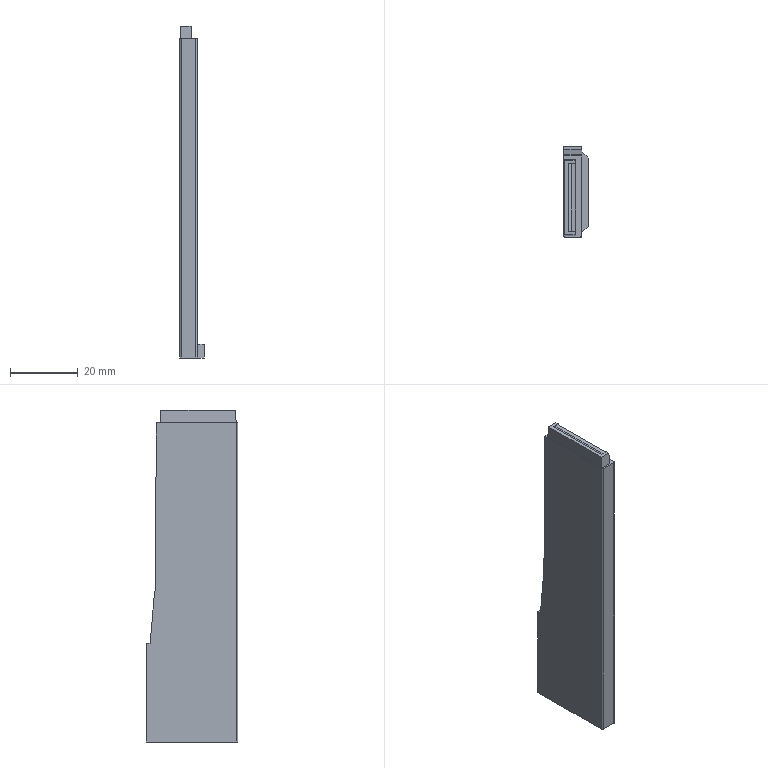Part | Creo | 1 solid | 28 faces | box 7.264 x 27.054 x 97.99 mm | volume 12954 mm3 | plane 25 | cylinder 3 | commonest cylinder face diameters 1 x3
STEP:
#1=CARTESIAN_POINT('',(0.,0.,0.));
#2=DIRECTION('',(0.,0.,1.));
#3=DIRECTION('',(1.,0.,0.));
#4=AXIS2_PLACEMENT_3D('',#1,#2,#3);
#5=CARTESIAN_POINT('',(19.635,62.146,-54.09));
#6=VERTEX_POINT('',#5);
#7=CARTESIAN_POINT('',(19.635,61.146,-54.09));
#8=VERTEX_POINT('',#7);
#9=CARTESIAN_POINT('',(19.635,62.146,-54.09));
#10=DIRECTION('',(0.,-1.,0.));
#11=VECTOR('',#10,1.);
#12=LINE('',#9,#11);
#13=EDGE_CURVE('',#6,#8,#12,.T.);
#14=ORIENTED_EDGE('',*,*,#13,.T.);
#15=CARTESIAN_POINT('',(19.635,61.146,40.081));
#16=VERTEX_POINT('',#15);
#17=CARTESIAN_POINT('',(19.635,61.146,-54.09));
#18=DIRECTION('',(0.,0.,1.));
#19=VECTOR('',#18,94.171);
#20=LINE('',#17,#19);
#21=EDGE_CURVE('',#8,#16,#20,.T.);
#22=ORIENTED_EDGE('',*,*,#21,.T.);
#23=CARTESIAN_POINT('',(19.635,84.661,40.081));
#24=VERTEX_POINT('',#23);
#25=CARTESIAN_POINT('',(19.635,61.146,40.081));
#26=DIRECTION('',(0.,1.,0.));
#27=VECTOR('',#26,23.515);
#28=LINE('',#25,#27);
#29=EDGE_CURVE('',#16,#24,#28,.T.);
#30=ORIENTED_EDGE('',*,*,#29,.T.);
#31=CARTESIAN_POINT('',(19.635,85.096,-9.767));
#32=VERTEX_POINT('',#31);
#33=CARTESIAN_POINT('',(19.635,85.096,-9.767));
#34=DIRECTION('',(0.,-0.008727,1.));
#35=VECTOR('',#34,49.85);
#36=LINE('',#33,#35);
#37=EDGE_CURVE('',#32,#24,#36,.T.);
#38=ORIENTED_EDGE('',*,*,#37,.F.);
#39=CARTESIAN_POINT('',(19.635,85.218,-9.767));
#40=VERTEX_POINT('',#39);
#41=CARTESIAN_POINT('',(19.635,85.218,-9.767));
#42=DIRECTION('',(0.,-1.,0.));
#43=VECTOR('',#42,0.1217);
#44=LINE('',#41,#43);
#45=EDGE_CURVE('',#40,#32,#44,.T.);
#46=ORIENTED_EDGE('',*,*,#45,.F.);
#47=CARTESIAN_POINT('',(19.635,86.547,-24.967));
#48=VERTEX_POINT('',#47);
#49=CARTESIAN_POINT('',(19.635,86.547,-24.967));
#50=DIRECTION('',(0.,-0.08716,0.9962));
#51=VECTOR('',#50,15.258);
#52=LINE('',#49,#51);
#53=EDGE_CURVE('',#48,#40,#52,.T.);
#54=ORIENTED_EDGE('',*,*,#53,.F.);
#55=CARTESIAN_POINT('',(19.635,87.2,-24.967));
#56=VERTEX_POINT('',#55);
#57=CARTESIAN_POINT('',(19.635,87.2,-24.967));
#58=DIRECTION('',(0.,-1.,0.));
#59=VECTOR('',#58,0.6527);
#60=LINE('',#57,#59);
#61=EDGE_CURVE('',#56,#48,#60,.T.);
#62=ORIENTED_EDGE('',*,*,#61,.F.);
#63=CARTESIAN_POINT('',(19.635,87.2,-54.09));
#64=VERTEX_POINT('',#63);
#65=CARTESIAN_POINT('',(19.635,87.2,-24.967));
#66=DIRECTION('',(0.,0.,-1.));
#67=VECTOR('',#66,29.123);
#68=LINE('',#65,#67);
#69=EDGE_CURVE('',#56,#64,#68,.T.);
#70=ORIENTED_EDGE('',*,*,#69,.T.);
#71=CARTESIAN_POINT('',(19.635,86.2,-54.09));
#72=VERTEX_POINT('',#71);
#73=CARTESIAN_POINT('',(19.635,87.2,-54.09));
#74=DIRECTION('',(0.,-1.,0.));
#75=VECTOR('',#74,1.);
#76=LINE('',#73,#75);
#77=EDGE_CURVE('',#64,#72,#76,.T.);
#78=ORIENTED_EDGE('',*,*,#77,.T.);
#79=CARTESIAN_POINT('',(19.635,86.2,-50.09));
#80=VERTEX_POINT('',#79);
#81=CARTESIAN_POINT('',(19.635,86.2,-54.09));
#82=DIRECTION('',(0.,0.,1.));
#83=VECTOR('',#82,4.);
#84=LINE('',#81,#83);
#85=EDGE_CURVE('',#72,#80,#84,.T.);
#86=ORIENTED_EDGE('',*,*,#85,.T.);
#87=CARTESIAN_POINT('',(19.635,62.146,-50.09));
#88=VERTEX_POINT('',#87);
#89=CARTESIAN_POINT('',(19.635,86.2,-50.09));
#90=DIRECTION('',(0.,-1.,0.));
#91=VECTOR('',#90,24.054);
#92=LINE('',#89,#91);
#93=EDGE_CURVE('',#80,#88,#92,.T.);
#94=ORIENTED_EDGE('',*,*,#93,.T.);
#95=CARTESIAN_POINT('',(19.635,62.146,-50.09));
#96=DIRECTION('',(0.,0.,-1.));
#97=VECTOR('',#96,4.);
#98=LINE('',#95,#97);
#99=EDGE_CURVE('',#88,#6,#98,.T.);
#100=ORIENTED_EDGE('',*,*,#99,.T.);
#101=EDGE_LOOP('',(#14,#22,#30,#38,#46,#54,#62,#70,#78,#86,#94,#100));
#102=FACE_OUTER_BOUND('',#101,.F.);
#103=CARTESIAN_POINT('',(19.635,60.646,75.91));
#104=DIRECTION('',(-1.,0.,0.));
#105=DIRECTION('',(0.,-1.,0.));
#106=AXIS2_PLACEMENT_3D('',#103,#104,#105);
#107=PLANE('',#106);
#108=ADVANCED_FACE('',(#102),#107,.F.);
#109=ORIENTED_EDGE('',*,*,#77,.F.);
#110=CARTESIAN_POINT('',(19.135,87.7,-54.09));
#111=VERTEX_POINT('',#110);
#112=CARTESIAN_POINT('',(19.135,87.2,-54.09));
#113=DIRECTION('',(0.,0.,-1.));
#114=DIRECTION('',(0.,1.,0.));
#115=AXIS2_PLACEMENT_3D('',#112,#113,#114);
#116=CIRCLE('',#115,0.5);
#117=EDGE_CURVE('',#111,#64,#116,.T.);
#118=ORIENTED_EDGE('',*,*,#117,.F.);
#119=CARTESIAN_POINT('',(14.371,87.7,-54.09));
#120=VERTEX_POINT('',#119);
#121=CARTESIAN_POINT('',(14.371,87.7,-54.09));
#122=DIRECTION('',(1.,0.,0.));
#123=VECTOR('',#122,4.764);
#124=LINE('',#121,#123);
#125=EDGE_CURVE('',#120,#111,#124,.T.);
#126=ORIENTED_EDGE('',*,*,#125,.F.);
#127=CARTESIAN_POINT('',(14.371,61.146,-54.09));
#128=VERTEX_POINT('',#127);
#129=CARTESIAN_POINT('',(14.371,61.146,-54.09));
#130=DIRECTION('',(0.,1.,0.));
#131=VECTOR('',#130,26.554);
#132=LINE('',#129,#131);
#133=EDGE_CURVE('',#128,#120,#132,.T.);
#134=ORIENTED_EDGE('',*,*,#133,.F.);
#135=CARTESIAN_POINT('',(14.871,60.646,-54.09));
#136=VERTEX_POINT('',#135);
#137=CARTESIAN_POINT('',(14.871,61.146,-54.09));
#138=DIRECTION('',(0.,0.,-1.));
#139=DIRECTION('',(0.,-1.,0.));
#140=AXIS2_PLACEMENT_3D('',#137,#138,#139);
#141=CIRCLE('',#140,0.5);
#142=EDGE_CURVE('',#136,#128,#141,.T.);
#143=ORIENTED_EDGE('',*,*,#142,.F.);
#144=CARTESIAN_POINT('',(19.135,60.646,-54.09));
#145=VERTEX_POINT('',#144);
#146=CARTESIAN_POINT('',(19.135,60.646,-54.09));
#147=DIRECTION('',(-1.,0.,0.));
#148=VECTOR('',#147,4.264);
#149=LINE('',#146,#148);
#150=EDGE_CURVE('',#145,#136,#149,.T.);
#151=ORIENTED_EDGE('',*,*,#150,.F.);
#152=CARTESIAN_POINT('',(19.135,61.146,-54.09));
#153=DIRECTION('',(0.,0.,-1.));
#154=DIRECTION('',(1.,0.,0.));
#155=AXIS2_PLACEMENT_3D('',#152,#153,#154);
#156=CIRCLE('',#155,0.5);
#157=EDGE_CURVE('',#8,#145,#156,.T.);
#158=ORIENTED_EDGE('',*,*,#157,.F.);
#159=ORIENTED_EDGE('',*,*,#13,.F.);
#160=CARTESIAN_POINT('',(21.635,64.146,-54.09));
#161=VERTEX_POINT('',#160);
#162=CARTESIAN_POINT('',(21.635,64.146,-54.09));
#163=DIRECTION('',(-0.7071,-0.7071,0.));
#164=VECTOR('',#163,2.828);
#165=LINE('',#162,#164);
#166=EDGE_CURVE('',#161,#6,#165,.T.);
#167=ORIENTED_EDGE('',*,*,#166,.F.);
#168=CARTESIAN_POINT('',(21.635,84.2,-54.09));
#169=VERTEX_POINT('',#168);
#170=CARTESIAN_POINT('',(21.635,84.2,-54.09));
#171=DIRECTION('',(0.,-1.,0.));
#172=VECTOR('',#171,20.054);
#173=LINE('',#170,#172);
#174=EDGE_CURVE('',#169,#161,#173,.T.);
#175=ORIENTED_EDGE('',*,*,#174,.F.);
#176=CARTESIAN_POINT('',(19.635,86.2,-54.09));
#177=DIRECTION('',(0.7071,-0.7071,0.));
#178=VECTOR('',#177,2.828);
#179=LINE('',#176,#178);
#180=EDGE_CURVE('',#72,#169,#179,.T.);
#181=ORIENTED_EDGE('',*,*,#180,.F.);
#182=EDGE_LOOP('',(#109,#118,#126,#134,#143,#151,#158,#159,#167,#175,#181));
#183=FACE_OUTER_BOUND('',#182,.F.);
#184=CARTESIAN_POINT('',(0.,0.,-54.09));
#185=DIRECTION('',(0.,0.,-1.));
#186=DIRECTION('',(-1.,0.,0.));
#187=AXIS2_PLACEMENT_3D('',#184,#185,#186);
#188=PLANE('',#187);
#189=ADVANCED_FACE('',(#183),#188,.T.);
#190=CARTESIAN_POINT('',(19.135,87.7,-24.967));
#191=VERTEX_POINT('',#190);
#192=CARTESIAN_POINT('',(19.135,87.2,-24.967));
#193=DIRECTION('',(0.,0.,1.));
#194=DIRECTION('',(1.,0.,0.));
#195=AXIS2_PLACEMENT_3D('',#192,#193,#194);
#196=CIRCLE('',#195,0.5);
#197=EDGE_CURVE('',#56,#191,#196,.T.);
#198=ORIENTED_EDGE('',*,*,#197,.T.);
#199=CARTESIAN_POINT('',(19.135,87.7,-54.09));
#200=DIRECTION('',(0.,0.,1.));
#201=VECTOR('',#200,29.123);
#202=LINE('',#199,#201);
#203=EDGE_CURVE('',#111,#191,#202,.T.);
#204=ORIENTED_EDGE('',*,*,#203,.F.);
#205=ORIENTED_EDGE('',*,*,#117,.T.);
#206=ORIENTED_EDGE('',*,*,#69,.F.);
#207=EDGE_LOOP('',(#198,#204,#205,#206));
#208=FACE_OUTER_BOUND('',#207,.F.);
#209=CARTESIAN_POINT('',(19.135,87.2,75.91));
#210=DIRECTION('',(0.,0.,-1.));
#211=DIRECTION('',(-1.,0.,0.));
#212=AXIS2_PLACEMENT_3D('',#209,#210,#211);
#213=CYLINDRICAL_SURFACE('',#212,0.5);
#214=ADVANCED_FACE('',(#208),#213,.T.);
#215=ORIENTED_EDGE('',*,*,#61,.T.);
#216=CARTESIAN_POINT('',(14.371,86.547,-24.967));
#217=VERTEX_POINT('',#216);
#218=CARTESIAN_POINT('',(14.371,86.547,-24.967));
#219=DIRECTION('',(1.,0.,0.));
#220=VECTOR('',#219,5.264);
#221=LINE('',#218,#220);
#222=EDGE_CURVE('',#217,#48,#221,.T.);
#223=ORIENTED_EDGE('',*,*,#222,.F.);
#224=CARTESIAN_POINT('',(14.371,87.7,-24.967));
#225=VERTEX_POINT('',#224);
#226=CARTESIAN_POINT('',(14.371,87.7,-24.967));
#227=DIRECTION('',(0.,-1.,0.));
#228=VECTOR('',#227,1.153);
#229=LINE('',#226,#228);
#230=EDGE_CURVE('',#225,#217,#229,.T.);
#231=ORIENTED_EDGE('',*,*,#230,.F.);
#232=CARTESIAN_POINT('',(14.371,87.7,-24.967));
#233=DIRECTION('',(1.,0.,0.));
#234=VECTOR('',#233,4.764);
#235=LINE('',#232,#234);
#236=EDGE_CURVE('',#225,#191,#235,.T.);
#237=ORIENTED_EDGE('',*,*,#236,.T.);
#238=ORIENTED_EDGE('',*,*,#197,.F.);
#239=EDGE_LOOP('',(#215,#223,#231,#237,#238));
#240=FACE_OUTER_BOUND('',#239,.F.);
#241=CARTESIAN_POINT('',(-0.07825,93.118,-24.967));
#242=DIRECTION('',(0.,0.,-1.));
#243=DIRECTION('',(0.,-1.,0.));
#244=AXIS2_PLACEMENT_3D('',#241,#242,#243);
#245=PLANE('',#244);
#246=ADVANCED_FACE('',(#240),#245,.F.);
#247=CARTESIAN_POINT('',(14.371,85.218,-9.767));
#248=VERTEX_POINT('',#247);
#249=CARTESIAN_POINT('',(14.371,85.218,-9.767));
#250=DIRECTION('',(1.,0.,0.));
#251=VECTOR('',#250,5.264);
#252=LINE('',#249,#251);
#253=EDGE_CURVE('',#248,#40,#252,.T.);
#254=ORIENTED_EDGE('',*,*,#253,.F.);
#255=CARTESIAN_POINT('',(14.371,85.218,-9.767));
#256=DIRECTION('',(0.,0.08716,-0.9962));
#257=VECTOR('',#256,15.258);
#258=LINE('',#255,#257);
#259=EDGE_CURVE('',#248,#217,#258,.T.);
#260=ORIENTED_EDGE('',*,*,#259,.T.);
#261=ORIENTED_EDGE('',*,*,#222,.T.);
#262=ORIENTED_EDGE('',*,*,#53,.T.);
#263=EDGE_LOOP('',(#254,#260,#261,#262));
#264=FACE_OUTER_BOUND('',#263,.F.);
#265=CARTESIAN_POINT('',(-0.07825,85.218,-9.767));
#266=DIRECTION('',(0.,-0.9962,-0.08716));
#267=DIRECTION('',(0.,-0.08716,0.9962));
#268=AXIS2_PLACEMENT_3D('',#265,#266,#267);
#269=PLANE('',#268);
#270=ADVANCED_FACE('',(#264),#269,.F.);
#271=CARTESIAN_POINT('',(14.371,85.096,-9.767));
#272=VERTEX_POINT('',#271);
#273=CARTESIAN_POINT('',(14.371,85.096,-9.767));
#274=DIRECTION('',(1.,0.,0.));
#275=VECTOR('',#274,5.264);
#276=LINE('',#273,#275);
#277=EDGE_CURVE('',#272,#32,#276,.T.);
#278=ORIENTED_EDGE('',*,*,#277,.F.);
#279=CARTESIAN_POINT('',(14.371,85.218,-9.767));
#280=DIRECTION('',(0.,-1.,0.));
#281=VECTOR('',#280,0.1217);
#282=LINE('',#279,#281);
#283=EDGE_CURVE('',#248,#272,#282,.T.);
#284=ORIENTED_EDGE('',*,*,#283,.F.);
#285=ORIENTED_EDGE('',*,*,#253,.T.);
#286=ORIENTED_EDGE('',*,*,#45,.T.);
#287=EDGE_LOOP('',(#278,#284,#285,#286));
#288=FACE_OUTER_BOUND('',#287,.F.);
#289=CARTESIAN_POINT('',(-0.07825,87.525,-9.767));
#290=DIRECTION('',(0.,0.,-1.));
#291=DIRECTION('',(0.,-1.,0.));
#292=AXIS2_PLACEMENT_3D('',#289,#290,#291);
#293=PLANE('',#292);
#294=ADVANCED_FACE('',(#288),#293,.F.);
#295=CARTESIAN_POINT('',(14.371,84.661,40.081));
#296=VERTEX_POINT('',#295);
#297=CARTESIAN_POINT('',(14.371,84.661,40.081));
#298=DIRECTION('',(1.,0.,0.));
#299=VECTOR('',#298,5.264);
#300=LINE('',#297,#299);
#301=EDGE_CURVE('',#296,#24,#300,.T.);
#302=ORIENTED_EDGE('',*,*,#301,.F.);
#303=CARTESIAN_POINT('',(14.371,84.661,40.081));
#304=DIRECTION('',(0.,0.008727,-1.));
#305=VECTOR('',#304,49.85);
#306=LINE('',#303,#305);
#307=EDGE_CURVE('',#296,#272,#306,.T.);
#308=ORIENTED_EDGE('',*,*,#307,.T.);
#309=ORIENTED_EDGE('',*,*,#277,.T.);
#310=ORIENTED_EDGE('',*,*,#37,.T.);
#311=EDGE_LOOP('',(#302,#308,#309,#310));
#312=FACE_OUTER_BOUND('',#311,.F.);
#313=CARTESIAN_POINT('',(31.073,85.013,-0.2195));
#314=DIRECTION('',(0.,-1.,-0.008727));
#315=DIRECTION('',(1.,0.,0.));
#316=AXIS2_PLACEMENT_3D('',#313,#314,#315);
#317=PLANE('',#316);
#318=ADVANCED_FACE('',(#312),#317,.F.);
#319=CARTESIAN_POINT('',(14.871,60.646,40.081));
#320=VERTEX_POINT('',#319);
#321=CARTESIAN_POINT('',(19.135,60.646,40.081));
#322=VERTEX_POINT('',#321);
#323=CARTESIAN_POINT('',(14.871,60.646,40.081));
#324=DIRECTION('',(1.,0.,0.));
#325=VECTOR('',#324,4.264);
#326=LINE('',#323,#325);
#327=EDGE_CURVE('',#320,#322,#326,.T.);
#328=ORIENTED_EDGE('',*,*,#327,.F.);
#329=CARTESIAN_POINT('',(14.371,61.146,40.081));
#330=VERTEX_POINT('',#329);
#331=CARTESIAN_POINT('',(14.871,61.146,40.081));
#332=DIRECTION('',(0.,0.,1.));
#333=DIRECTION('',(-1.,0.,0.));
#334=AXIS2_PLACEMENT_3D('',#331,#332,#333);
#335=CIRCLE('',#334,0.5);
#336=EDGE_CURVE('',#330,#320,#335,.T.);
#337=ORIENTED_EDGE('',*,*,#336,.F.);
#338=CARTESIAN_POINT('',(14.371,61.146,40.081));
#339=DIRECTION('',(0.,1.,0.));
#340=VECTOR('',#339,23.515);
#341=LINE('',#338,#340);
#342=EDGE_CURVE('',#330,#296,#341,.T.);
#343=ORIENTED_EDGE('',*,*,#342,.T.);
#344=ORIENTED_EDGE('',*,*,#301,.T.);
#345=ORIENTED_EDGE('',*,*,#29,.F.);
#346=CARTESIAN_POINT('',(19.135,61.146,40.081));
#347=DIRECTION('',(0.,0.,1.));
#348=DIRECTION('',(0.,-1.,0.));
#349=AXIS2_PLACEMENT_3D('',#346,#347,#348);
#350=CIRCLE('',#349,0.5);
#351=EDGE_CURVE('',#322,#16,#350,.T.);
#352=ORIENTED_EDGE('',*,*,#351,.F.);
#353=EDGE_LOOP('',(#328,#337,#343,#344,#345,#352));
#354=FACE_OUTER_BOUND('',#353,.F.);
#355=CARTESIAN_POINT('',(14.471,83.604,40.081));
#356=VERTEX_POINT('',#355);
#357=CARTESIAN_POINT('',(17.921,83.604,40.081));
#358=VERTEX_POINT('',#357);
#359=CARTESIAN_POINT('',(14.471,83.604,40.081));
#360=DIRECTION('',(1.,0.,0.));
#361=VECTOR('',#360,3.45);
#362=LINE('',#359,#361);
#363=EDGE_CURVE('',#356,#358,#362,.T.);
#364=ORIENTED_EDGE('',*,*,#363,.F.);
#365=CARTESIAN_POINT('',(14.471,61.146,40.081));
#366=VERTEX_POINT('',#365);
#367=CARTESIAN_POINT('',(14.471,61.146,40.081));
#368=DIRECTION('',(0.,1.,0.));
#369=VECTOR('',#368,22.458);
#370=LINE('',#367,#369);
#371=EDGE_CURVE('',#366,#356,#370,.T.);
#372=ORIENTED_EDGE('',*,*,#371,.F.);
#373=CARTESIAN_POINT('',(17.921,61.146,40.081));
#374=VERTEX_POINT('',#373);
#375=CARTESIAN_POINT('',(17.921,61.146,40.081));
#376=DIRECTION('',(-1.,0.,0.));
#377=VECTOR('',#376,3.45);
#378=LINE('',#375,#377);
#379=EDGE_CURVE('',#374,#366,#378,.T.);
#380=ORIENTED_EDGE('',*,*,#379,.F.);
#381=CARTESIAN_POINT('',(17.921,61.146,40.081));
#382=DIRECTION('',(0.,1.,0.));
#383=VECTOR('',#382,22.458);
#384=LINE('',#381,#383);
#385=EDGE_CURVE('',#374,#358,#384,.T.);
#386=ORIENTED_EDGE('',*,*,#385,.T.);
#387=EDGE_LOOP('',(#364,#372,#380,#386));
#388=FACE_BOUND('',#387,.F.);
#389=CARTESIAN_POINT('',(-17.817,-88.35,40.081));
#390=DIRECTION('',(0.,0.,1.));
#391=DIRECTION('',(-1.,0.,0.));
#392=AXIS2_PLACEMENT_3D('',#389,#390,#391);
#393=PLANE('',#392);
#394=ADVANCED_FACE('',(#354,#388),#393,.T.);
#395=CARTESIAN_POINT('',(19.135,60.646,40.081));
#396=DIRECTION('',(0.,0.,-1.));
#397=VECTOR('',#396,94.171);
#398=LINE('',#395,#397);
#399=EDGE_CURVE('',#322,#145,#398,.T.);
#400=ORIENTED_EDGE('',*,*,#399,.T.);
#401=ORIENTED_EDGE('',*,*,#150,.T.);
#402=CARTESIAN_POINT('',(14.871,60.646,-54.09));
#403=DIRECTION('',(0.,0.,1.));
#404=VECTOR('',#403,94.171);
#405=LINE('',#402,#404);
#406=EDGE_CURVE('',#136,#320,#405,.T.);
#407=ORIENTED_EDGE('',*,*,#406,.T.);
#408=ORIENTED_EDGE('',*,*,#327,.T.);
#409=EDGE_LOOP('',(#400,#401,#407,#408));
#410=FACE_OUTER_BOUND('',#409,.F.);
#411=CARTESIAN_POINT('',(14.371,60.646,75.91));
#412=DIRECTION('',(0.,1.,0.));
#413=DIRECTION('',(-1.,0.,0.));
#414=AXIS2_PLACEMENT_3D('',#411,#412,#413);
#415=PLANE('',#414);
#416=ADVANCED_FACE('',(#410),#415,.F.);
#417=ORIENTED_EDGE('',*,*,#351,.T.);
#418=ORIENTED_EDGE('',*,*,#21,.F.);
#419=ORIENTED_EDGE('',*,*,#157,.T.);
#420=ORIENTED_EDGE('',*,*,#399,.F.);
#421=EDGE_LOOP('',(#417,#418,#419,#420));
#422=FACE_OUTER_BOUND('',#421,.F.);
#423=CARTESIAN_POINT('',(19.135,61.146,75.91));
#424=DIRECTION('',(0.,0.,-1.));
#425=DIRECTION('',(-1.,0.,0.));
#426=AXIS2_PLACEMENT_3D('',#423,#424,#425);
#427=CYLINDRICAL_SURFACE('',#426,0.5);
#428=ADVANCED_FACE('',(#422),#427,.T.);
#429=ORIENTED_EDGE('',*,*,#336,.T.);
#430=ORIENTED_EDGE('',*,*,#406,.F.);
#431=ORIENTED_EDGE('',*,*,#142,.T.);
#432=CARTESIAN_POINT('',(14.371,61.146,40.081));
#433=DIRECTION('',(0.,0.,-1.));
#434=VECTOR('',#433,94.171);
#435=LINE('',#432,#434);
#436=EDGE_CURVE('',#330,#128,#435,.T.);
#437=ORIENTED_EDGE('',*,*,#436,.F.);
#438=EDGE_LOOP('',(#429,#430,#431,#437));
#439=FACE_OUTER_BOUND('',#438,.F.);
#440=CARTESIAN_POINT('',(14.871,61.146,75.91));
#441=DIRECTION('',(0.,0.,-1.));
#442=DIRECTION('',(-1.,0.,0.));
#443=AXIS2_PLACEMENT_3D('',#440,#441,#442);
#444=CYLINDRICAL_SURFACE('',#443,0.5);
#445=ADVANCED_FACE('',(#439),#444,.T.);
#446=ORIENTED_EDGE('',*,*,#307,.F.);
#447=ORIENTED_EDGE('',*,*,#342,.F.);
#448=ORIENTED_EDGE('',*,*,#436,.T.);
#449=ORIENTED_EDGE('',*,*,#133,.T.);
#450=CARTESIAN_POINT('',(14.371,87.7,-54.09));
#451=DIRECTION('',(0.,0.,1.));
#452=VECTOR('',#451,29.123);
#453=LINE('',#450,#452);
#454=EDGE_CURVE('',#120,#225,#453,.T.);
#455=ORIENTED_EDGE('',*,*,#454,.T.);
#456=ORIENTED_EDGE('',*,*,#230,.T.);
#457=ORIENTED_EDGE('',*,*,#259,.F.);
#458=ORIENTED_EDGE('',*,*,#283,.T.);
#459=EDGE_LOOP('',(#446,#447,#448,#449,#455,#456,#457,#458));
#460=FACE_OUTER_BOUND('',#459,.F.);
#461=CARTESIAN_POINT('',(14.371,76.162,68.91));
#462=DIRECTION('',(-1.,0.,0.));
#463=DIRECTION('',(0.,0.,1.));
#464=AXIS2_PLACEMENT_3D('',#461,#462,#463);
#465=PLANE('',#464);
#466=ADVANCED_FACE('',(#460),#465,.T.);
#467=ORIENTED_EDGE('',*,*,#236,.F.);
#468=ORIENTED_EDGE('',*,*,#454,.F.);
#469=ORIENTED_EDGE('',*,*,#125,.T.);
#470=ORIENTED_EDGE('',*,*,#203,.T.);
#471=EDGE_LOOP('',(#467,#468,#469,#470));
#472=FACE_OUTER_BOUND('',#471,.F.);
#473=CARTESIAN_POINT('',(19.635,87.7,75.91));
#474=DIRECTION('',(0.,-1.,0.));
#475=DIRECTION('',(0.,0.,-1.));
#476=AXIS2_PLACEMENT_3D('',#473,#474,#475);
#477=PLANE('',#476);
#478=ADVANCED_FACE('',(#472),#477,.F.);
#479=CARTESIAN_POINT('',(17.722,83.405,43.876));
#480=VERTEX_POINT('',#479);
#481=CARTESIAN_POINT('',(17.723,83.403,43.9));
#482=VERTEX_POINT('',#481);
#483=CARTESIAN_POINT('',(17.722,83.405,43.876));
#484=DIRECTION('',(0.03485,-0.0523,0.998));
#485=VECTOR('',#484,0.02412);
#486=LINE('',#483,#485);
#487=EDGE_CURVE('',#480,#482,#486,.T.);
#488=ORIENTED_EDGE('',*,*,#487,.T.);
#489=CARTESIAN_POINT('',(14.671,83.403,43.9));
#490=VERTEX_POINT('',#489);
#491=CARTESIAN_POINT('',(17.723,83.403,43.9));
#492=DIRECTION('',(-1.,0.,0.));
#493=VECTOR('',#492,3.052);
#494=LINE('',#491,#493);
#495=EDGE_CURVE('',#482,#490,#494,.T.);
#496=ORIENTED_EDGE('',*,*,#495,.T.);
#497=CARTESIAN_POINT('',(14.671,83.403,43.9));
#498=DIRECTION('',(-0.05226,0.05226,-0.9973));
#499=VECTOR('',#498,3.829);
#500=LINE('',#497,#499);
#501=EDGE_CURVE('',#490,#356,#500,.T.);
#502=ORIENTED_EDGE('',*,*,#501,.T.);
#503=ORIENTED_EDGE('',*,*,#363,.T.);
#504=CARTESIAN_POINT('',(17.921,83.604,40.081));
#505=DIRECTION('',(-0.05226,-0.05226,0.9973));
#506=VECTOR('',#505,3.805);
#507=LINE('',#504,#506);
#508=EDGE_CURVE('',#358,#480,#507,.T.);
#509=ORIENTED_EDGE('',*,*,#508,.T.);
#510=EDGE_LOOP('',(#488,#496,#502,#503,#509));
#511=FACE_OUTER_BOUND('',#510,.F.);
#512=CARTESIAN_POINT('',(21.275,83.43,43.398));
#513=DIRECTION('',(0.,0.9986,0.05234));
#514=DIRECTION('',(-1.,0.,0.));
#515=AXIS2_PLACEMENT_3D('',#512,#513,#514);
#516=PLANE('',#515);
#517=ADVANCED_FACE('',(#511),#516,.T.);
#518=CARTESIAN_POINT('',(17.723,82.5,43.9));
#519=VERTEX_POINT('',#518);
#520=CARTESIAN_POINT('',(17.723,82.5,43.9));
#521=DIRECTION('',(0.,1.,0.));
#522=VECTOR('',#521,0.9034);
#523=LINE('',#520,#522);
#524=EDGE_CURVE('',#519,#482,#523,.T.);
#525=ORIENTED_EDGE('',*,*,#524,.T.);
#526=ORIENTED_EDGE('',*,*,#487,.F.);
#527=CARTESIAN_POINT('',(17.722,82.498,43.876));
#528=VERTEX_POINT('',#527);
#529=CARTESIAN_POINT('',(17.722,82.498,43.876));
#530=DIRECTION('',(0.,1.,0.));
#531=VECTOR('',#530,0.9067);
#532=LINE('',#529,#531);
#533=EDGE_CURVE('',#528,#480,#532,.T.);
#534=ORIENTED_EDGE('',*,*,#533,.F.);
#535=CARTESIAN_POINT('',(17.723,82.5,43.9));
#536=DIRECTION('',(-0.03477,-0.0871,-0.9956));
#537=VECTOR('',#536,0.02417);
#538=LINE('',#535,#537);
#539=EDGE_CURVE('',#519,#528,#538,.T.);
#540=ORIENTED_EDGE('',*,*,#539,.F.);
#541=EDGE_LOOP('',(#525,#526,#534,#540));
#542=FACE_OUTER_BOUND('',#541,.F.);
#543=CARTESIAN_POINT('',(17.66,83.498,42.091));
#544=DIRECTION('',(-0.9994,0.,0.0349));
#545=DIRECTION('',(0.0349,0.,0.9994));
#546=AXIS2_PLACEMENT_3D('',#543,#544,#545);
#547=PLANE('',#546);
#548=ADVANCED_FACE('',(#542),#547,.F.);
#549=CARTESIAN_POINT('',(15.65,82.5,43.9));
#550=VERTEX_POINT('',#549);
#551=CARTESIAN_POINT('',(17.723,82.5,43.9));
#552=DIRECTION('',(-1.,0.,0.));
#553=VECTOR('',#552,2.073);
#554=LINE('',#551,#553);
#555=EDGE_CURVE('',#519,#550,#554,.T.);
#556=ORIENTED_EDGE('',*,*,#555,.T.);
#557=CARTESIAN_POINT('',(15.65,62.4,43.9));
#558=VERTEX_POINT('',#557);
#559=CARTESIAN_POINT('',(15.65,82.5,43.9));
#560=DIRECTION('',(0.,-1.,0.));
#561=VECTOR('',#560,20.1);
#562=LINE('',#559,#561);
#563=EDGE_CURVE('',#550,#558,#562,.T.);
#564=ORIENTED_EDGE('',*,*,#563,.T.);
#565=CARTESIAN_POINT('',(17.723,62.4,43.9));
#566=VERTEX_POINT('',#565);
#567=CARTESIAN_POINT('',(15.65,62.4,43.9));
#568=DIRECTION('',(1.,0.,0.));
#569=VECTOR('',#568,2.073);
#570=LINE('',#567,#569);
#571=EDGE_CURVE('',#558,#566,#570,.T.);
#572=ORIENTED_EDGE('',*,*,#571,.T.);
#573=CARTESIAN_POINT('',(17.723,61.346,43.9));
#574=VERTEX_POINT('',#573);
#575=CARTESIAN_POINT('',(17.723,61.346,43.9));
#576=DIRECTION('',(0.,1.,0.));
#577=VECTOR('',#576,1.054);
#578=LINE('',#575,#577);
#579=EDGE_CURVE('',#574,#566,#578,.T.);
#580=ORIENTED_EDGE('',*,*,#579,.F.);
#581=CARTESIAN_POINT('',(14.671,61.346,43.9));
#582=VERTEX_POINT('',#581);
#583=CARTESIAN_POINT('',(14.671,61.346,43.9));
#584=DIRECTION('',(1.,0.,0.));
#585=VECTOR('',#584,3.052);
#586=LINE('',#583,#585);
#587=EDGE_CURVE('',#582,#574,#586,.T.);
#588=ORIENTED_EDGE('',*,*,#587,.F.);
#589=CARTESIAN_POINT('',(14.671,83.403,43.9));
#590=DIRECTION('',(0.,-1.,0.));
#591=VECTOR('',#590,22.057);
#592=LINE('',#589,#591);
#593=EDGE_CURVE('',#490,#582,#592,.T.);
#594=ORIENTED_EDGE('',*,*,#593,.F.);
#595=ORIENTED_EDGE('',*,*,#495,.F.);
#596=ORIENTED_EDGE('',*,*,#524,.F.);
#597=EDGE_LOOP('',(#556,#564,#572,#580,#588,#594,#595,#596));
#598=FACE_OUTER_BOUND('',#597,.F.);
#599=CARTESIAN_POINT('',(-46.35,62.4,43.9));
#600=DIRECTION('',(0.,0.,-1.));
#601=DIRECTION('',(0.,-1.,0.));
#602=AXIS2_PLACEMENT_3D('',#599,#600,#601);
#603=PLANE('',#602);
#604=ADVANCED_FACE('',(#598),#603,.F.);
#605=ORIENTED_EDGE('',*,*,#555,.F.);
#606=ORIENTED_EDGE('',*,*,#539,.T.);
#607=CARTESIAN_POINT('',(17.74,82.469,43.548));
#608=VERTEX_POINT('',#607);
#609=CARTESIAN_POINT('',(17.722,82.498,43.876));
#610=DIRECTION('',(0.05214,-0.08704,-0.9948));
#611=VECTOR('',#610,0.3299);
#612=LINE('',#609,#611);
#613=EDGE_CURVE('',#528,#608,#612,.T.);
#614=ORIENTED_EDGE('',*,*,#613,.T.);
#615=CARTESIAN_POINT('',(16.566,82.469,43.548));
#616=VERTEX_POINT('',#615);
#617=CARTESIAN_POINT('',(16.566,82.469,43.548));
#618=DIRECTION('',(1.,0.,0.));
#619=VECTOR('',#618,1.174);
#620=LINE('',#617,#619);
#621=EDGE_CURVE('',#616,#608,#620,.T.);
#622=ORIENTED_EDGE('',*,*,#621,.F.);
#623=CARTESIAN_POINT('',(15.65,82.5,43.9));
#624=DIRECTION('',(0.9329,-0.03139,-0.3588));
#625=VECTOR('',#624,0.9817);
#626=LINE('',#623,#625);
#627=EDGE_CURVE('',#550,#616,#626,.T.);
#628=ORIENTED_EDGE('',*,*,#627,.F.);
#629=EDGE_LOOP('',(#605,#606,#614,#622,#628));
#630=FACE_OUTER_BOUND('',#629,.F.);
#631=CARTESIAN_POINT('',(-0.07825,82.5,43.9));
#632=DIRECTION('',(0.,0.9962,-0.08716));
#633=DIRECTION('',(0.,-0.08716,-0.9962));
#634=AXIS2_PLACEMENT_3D('',#631,#632,#633);
#635=PLANE('',#634);
#636=ADVANCED_FACE('',(#630),#635,.F.);
#637=ORIENTED_EDGE('',*,*,#508,.F.);
#638=ORIENTED_EDGE('',*,*,#385,.F.);
#639=CARTESIAN_POINT('',(17.722,61.345,43.876));
#640=VERTEX_POINT('',#639);
#641=CARTESIAN_POINT('',(17.722,61.345,43.876));
#642=DIRECTION('',(0.05226,-0.05226,-0.9973));
#643=VECTOR('',#642,3.805);
#644=LINE('',#641,#643);
#645=EDGE_CURVE('',#640,#374,#644,.T.);
#646=ORIENTED_EDGE('',*,*,#645,.F.);
#647=CARTESIAN_POINT('',(17.722,62.402,43.876));
#648=VERTEX_POINT('',#647);
#649=CARTESIAN_POINT('',(17.722,61.345,43.876));
#650=DIRECTION('',(0.,1.,0.));
#651=VECTOR('',#650,1.057);
#652=LINE('',#649,#651);
#653=EDGE_CURVE('',#640,#648,#652,.T.);
#654=ORIENTED_EDGE('',*,*,#653,.T.);
#655=CARTESIAN_POINT('',(17.74,62.431,43.548));
#656=VERTEX_POINT('',#655);
#657=CARTESIAN_POINT('',(17.74,62.431,43.548));
#658=DIRECTION('',(-0.05214,-0.08704,0.9948));
#659=VECTOR('',#658,0.3299);
#660=LINE('',#657,#659);
#661=EDGE_CURVE('',#656,#648,#660,.T.);
#662=ORIENTED_EDGE('',*,*,#661,.F.);
#663=CARTESIAN_POINT('',(17.74,62.431,43.548));
#664=DIRECTION('',(0.,1.,0.));
#665=VECTOR('',#664,20.038);
#666=LINE('',#663,#665);
#667=EDGE_CURVE('',#656,#608,#666,.T.);
#668=ORIENTED_EDGE('',*,*,#667,.T.);
#669=ORIENTED_EDGE('',*,*,#613,.F.);
#670=ORIENTED_EDGE('',*,*,#533,.T.);
#671=EDGE_LOOP('',(#637,#638,#646,#654,#662,#668,#669,#670));
#672=FACE_OUTER_BOUND('',#671,.F.);
#673=CARTESIAN_POINT('',(17.747,-90.96,43.402));
#674=DIRECTION('',(-0.9986,0.,-0.05234));
#675=DIRECTION('',(0.,-1.,0.));
#676=AXIS2_PLACEMENT_3D('',#673,#674,#675);
#677=PLANE('',#676);
#678=ADVANCED_FACE('',(#672),#677,.F.);
#679=ORIENTED_EDGE('',*,*,#645,.T.);
#680=ORIENTED_EDGE('',*,*,#379,.T.);
#681=CARTESIAN_POINT('',(14.671,61.346,43.9));
#682=DIRECTION('',(-0.05226,-0.05226,-0.9973));
#683=VECTOR('',#682,3.829);
#684=LINE('',#681,#683);
#685=EDGE_CURVE('',#582,#366,#684,.T.);
#686=ORIENTED_EDGE('',*,*,#685,.F.);
#687=ORIENTED_EDGE('',*,*,#587,.T.);
#688=CARTESIAN_POINT('',(17.722,61.345,43.876));
#689=DIRECTION('',(0.03485,0.0523,0.998));
#690=VECTOR('',#689,0.02412);
#691=LINE('',#688,#690);
#692=EDGE_CURVE('',#640,#574,#691,.T.);
#693=ORIENTED_EDGE('',*,*,#692,.F.);
#694=EDGE_LOOP('',(#679,#680,#686,#687,#693));
#695=FACE_OUTER_BOUND('',#694,.F.);
#696=CARTESIAN_POINT('',(11.03,61.32,43.398));
#697=DIRECTION('',(0.,-0.9986,0.05234));
#698=DIRECTION('',(1.,0.,0.));
#699=AXIS2_PLACEMENT_3D('',#696,#697,#698);
#700=PLANE('',#699);
#701=ADVANCED_FACE('',(#695),#700,.T.);
#702=ORIENTED_EDGE('',*,*,#685,.T.);
#703=ORIENTED_EDGE('',*,*,#371,.T.);
#704=ORIENTED_EDGE('',*,*,#501,.F.);
#705=ORIENTED_EDGE('',*,*,#593,.T.);
#706=EDGE_LOOP('',(#702,#703,#704,#705));
#707=FACE_OUTER_BOUND('',#706,.F.);
#708=CARTESIAN_POINT('',(14.645,87.044,43.398));
#709=DIRECTION('',(-0.9986,0.,0.05234));
#710=DIRECTION('',(0.,-1.,0.));
#711=AXIS2_PLACEMENT_3D('',#708,#709,#710);
#712=PLANE('',#711);
#713=ADVANCED_FACE('',(#707),#712,.T.);
#714=ORIENTED_EDGE('',*,*,#579,.T.);
#715=CARTESIAN_POINT('',(17.723,62.4,43.9));
#716=DIRECTION('',(-0.03477,0.0871,-0.9956));
#717=VECTOR('',#716,0.02417);
#718=LINE('',#715,#717);
#719=EDGE_CURVE('',#566,#648,#718,.T.);
#720=ORIENTED_EDGE('',*,*,#719,.T.);
#721=ORIENTED_EDGE('',*,*,#653,.F.);
#722=ORIENTED_EDGE('',*,*,#692,.T.);
#723=EDGE_LOOP('',(#714,#720,#721,#722));
#724=FACE_OUTER_BOUND('',#723,.F.);
#725=CARTESIAN_POINT('',(17.66,-62.152,42.091));
#726=DIRECTION('',(-0.9994,0.,0.0349));
#727=DIRECTION('',(0.0349,0.,0.9994));
#728=AXIS2_PLACEMENT_3D('',#725,#726,#727);
#729=PLANE('',#728);
#730=ADVANCED_FACE('',(#724),#729,.F.);
#731=ORIENTED_EDGE('',*,*,#719,.F.);
#732=ORIENTED_EDGE('',*,*,#571,.F.);
#733=CARTESIAN_POINT('',(16.566,62.431,43.548));
#734=VERTEX_POINT('',#733);
#735=CARTESIAN_POINT('',(15.65,62.4,43.9));
#736=DIRECTION('',(0.9329,0.03139,-0.3588));
#737=VECTOR('',#736,0.9817);
#738=LINE('',#735,#737);
#739=EDGE_CURVE('',#558,#734,#738,.T.);
#740=ORIENTED_EDGE('',*,*,#739,.T.);
#741=CARTESIAN_POINT('',(16.566,62.431,43.548));
#742=DIRECTION('',(1.,0.,0.));
#743=VECTOR('',#742,1.174);
#744=LINE('',#741,#743);
#745=EDGE_CURVE('',#734,#656,#744,.T.);
#746=ORIENTED_EDGE('',*,*,#745,.T.);
#747=ORIENTED_EDGE('',*,*,#661,.T.);
#748=EDGE_LOOP('',(#731,#732,#740,#746,#747));
#749=FACE_OUTER_BOUND('',#748,.F.);
#750=CARTESIAN_POINT('',(-0.07825,62.4,43.9));
#751=DIRECTION('',(0.,-0.9962,-0.08716));
#752=DIRECTION('',(0.,-0.08716,0.9962));
#753=AXIS2_PLACEMENT_3D('',#750,#751,#752);
#754=PLANE('',#753);
#755=ADVANCED_FACE('',(#749),#754,.F.);
#756=CARTESIAN_POINT('',(16.566,82.469,43.548));
#757=DIRECTION('',(0.,-1.,0.));
#758=VECTOR('',#757,20.038);
#759=LINE('',#756,#758);
#760=EDGE_CURVE('',#616,#734,#759,.T.);
#761=ORIENTED_EDGE('',*,*,#760,.T.);
#762=ORIENTED_EDGE('',*,*,#739,.F.);
#763=ORIENTED_EDGE('',*,*,#563,.F.);
#764=ORIENTED_EDGE('',*,*,#627,.T.);
#765=EDGE_LOOP('',(#761,#762,#763,#764));
#766=FACE_OUTER_BOUND('',#765,.F.);
#767=CARTESIAN_POINT('',(15.65,82.5,43.9));
#768=DIRECTION('',(0.359,0.,0.9333));
#769=DIRECTION('',(-0.9333,0.,0.359));
#770=AXIS2_PLACEMENT_3D('',#767,#768,#769);
#771=PLANE('',#770);
#772=ADVANCED_FACE('',(#766),#771,.T.);
#773=ORIENTED_EDGE('',*,*,#745,.F.);
#774=ORIENTED_EDGE('',*,*,#760,.F.);
#775=ORIENTED_EDGE('',*,*,#621,.T.);
#776=ORIENTED_EDGE('',*,*,#667,.F.);
#777=EDGE_LOOP('',(#773,#774,#775,#776));
#778=FACE_OUTER_BOUND('',#777,.F.);
#779=CARTESIAN_POINT('',(16.956,82.5,43.548));
#780=DIRECTION('',(0.,0.,1.));
#781=DIRECTION('',(-1.,0.,0.));
#782=AXIS2_PLACEMENT_3D('',#779,#780,#781);
#783=PLANE('',#782);
#784=ADVANCED_FACE('',(#778),#783,.T.);
#785=ORIENTED_EDGE('',*,*,#166,.T.);
#786=ORIENTED_EDGE('',*,*,#99,.F.);
#787=CARTESIAN_POINT('',(21.635,64.146,-50.09));
#788=VERTEX_POINT('',#787);
#789=CARTESIAN_POINT('',(19.635,62.146,-50.09));
#790=DIRECTION('',(0.7071,0.7071,0.));
#791=VECTOR('',#790,2.828);
#792=LINE('',#789,#791);
#793=EDGE_CURVE('',#88,#788,#792,.T.);
#794=ORIENTED_EDGE('',*,*,#793,.T.);
#795=CARTESIAN_POINT('',(21.635,64.146,-54.09));
#796=DIRECTION('',(0.,0.,1.));
#797=VECTOR('',#796,4.);
#798=LINE('',#795,#797);
#799=EDGE_CURVE('',#161,#788,#798,.T.);
#800=ORIENTED_EDGE('',*,*,#799,.F.);
#801=EDGE_LOOP('',(#785,#786,#794,#800));
#802=FACE_OUTER_BOUND('',#801,.F.);
#803=CARTESIAN_POINT('',(19.635,62.146,-54.09));
#804=DIRECTION('',(-0.7071,0.7071,0.));
#805=DIRECTION('',(0.,0.,1.));
#806=AXIS2_PLACEMENT_3D('',#803,#804,#805);
#807=PLANE('',#806);
#808=ADVANCED_FACE('',(#802),#807,.F.);
#809=CARTESIAN_POINT('',(21.635,84.2,-50.09));
#810=VERTEX_POINT('',#809);
#811=CARTESIAN_POINT('',(21.635,64.146,-50.09));
#812=DIRECTION('',(0.,1.,0.));
#813=VECTOR('',#812,20.054);
#814=LINE('',#811,#813);
#815=EDGE_CURVE('',#788,#810,#814,.T.);
#816=ORIENTED_EDGE('',*,*,#815,.F.);
#817=ORIENTED_EDGE('',*,*,#793,.F.);
#818=ORIENTED_EDGE('',*,*,#93,.F.);
#819=CARTESIAN_POINT('',(21.635,84.2,-50.09));
#820=DIRECTION('',(-0.7071,0.7071,0.));
#821=VECTOR('',#820,2.828);
#822=LINE('',#819,#821);
#823=EDGE_CURVE('',#810,#80,#822,.T.);
#824=ORIENTED_EDGE('',*,*,#823,.F.);
#825=EDGE_LOOP('',(#816,#817,#818,#824));
#826=FACE_OUTER_BOUND('',#825,.F.);
#827=CARTESIAN_POINT('',(20.135,74.173,-50.09));
#828=DIRECTION('',(0.,0.,1.));
#829=DIRECTION('',(1.,0.,0.));
#830=AXIS2_PLACEMENT_3D('',#827,#828,#829);
#831=PLANE('',#830);
#832=ADVANCED_FACE('',(#826),#831,.T.);
#833=ORIENTED_EDGE('',*,*,#174,.T.);
#834=ORIENTED_EDGE('',*,*,#799,.T.);
#835=ORIENTED_EDGE('',*,*,#815,.T.);
#836=CARTESIAN_POINT('',(21.635,84.2,-50.09));
#837=DIRECTION('',(0.,0.,-1.));
#838=VECTOR('',#837,4.);
#839=LINE('',#836,#838);
#840=EDGE_CURVE('',#810,#169,#839,.T.);
#841=ORIENTED_EDGE('',*,*,#840,.T.);
#842=EDGE_LOOP('',(#833,#834,#835,#841));
#843=FACE_OUTER_BOUND('',#842,.F.);
#844=CARTESIAN_POINT('',(21.635,74.173,-54.09));
#845=DIRECTION('',(1.,0.,0.));
#846=DIRECTION('',(0.,0.,-1.));
#847=AXIS2_PLACEMENT_3D('',#844,#845,#846);
#848=PLANE('',#847);
#849=ADVANCED_FACE('',(#843),#848,.T.);
#850=ORIENTED_EDGE('',*,*,#180,.T.);
#851=ORIENTED_EDGE('',*,*,#840,.F.);
#852=ORIENTED_EDGE('',*,*,#823,.T.);
#853=ORIENTED_EDGE('',*,*,#85,.F.);
#854=EDGE_LOOP('',(#850,#851,#852,#853));
#855=FACE_OUTER_BOUND('',#854,.F.);
#856=CARTESIAN_POINT('',(21.635,84.2,-54.09));
#857=DIRECTION('',(-0.7071,-0.7071,0.));
#858=DIRECTION('',(0.,0.,1.));
#859=AXIS2_PLACEMENT_3D('',#856,#857,#858);
#860=PLANE('',#859);
#861=ADVANCED_FACE('',(#855),#860,.F.);
#862=CLOSED_SHELL('',(#108,#189,#214,#246,#270,#294,#318,#394,#416,#428,#445,#466,#478,#517,#548,#604,#636,#678,#701,#713,#730,#755,#772,#784,#808,#832,#849,#861));
#863=MANIFOLD_SOLID_BREP('',#862);
#864=(LENGTH_UNIT()NAMED_UNIT(*)SI_UNIT(.MILLI.,.METRE.));
#865=UNCERTAINTY_MEASURE_WITH_UNIT(LENGTH_MEASURE(0.01019),#864,'','');
#866=(NAMED_UNIT(*)PLANE_ANGLE_UNIT()SI_UNIT($,.RADIAN.));
#867=PLANE_ANGLE_MEASURE_WITH_UNIT(PLANE_ANGLE_MEASURE(0.01745),#866);
#868=(CONVERSION_BASED_UNIT('DEGREE',#867)NAMED_UNIT(*)PLANE_ANGLE_UNIT());
#869=(NAMED_UNIT(*)SI_UNIT($,.STERADIAN.)SOLID_ANGLE_UNIT());
#870=(GEOMETRIC_REPRESENTATION_CONTEXT(3)GLOBAL_UNCERTAINTY_ASSIGNED_CONTEXT((#865))GLOBAL_UNIT_ASSIGNED_CONTEXT((#864,#868,#869))REPRESENTATION_CONTEXT('',''));
#871=ADVANCED_BREP_SHAPE_REPRESENTATION('',(#4,#863),#870);